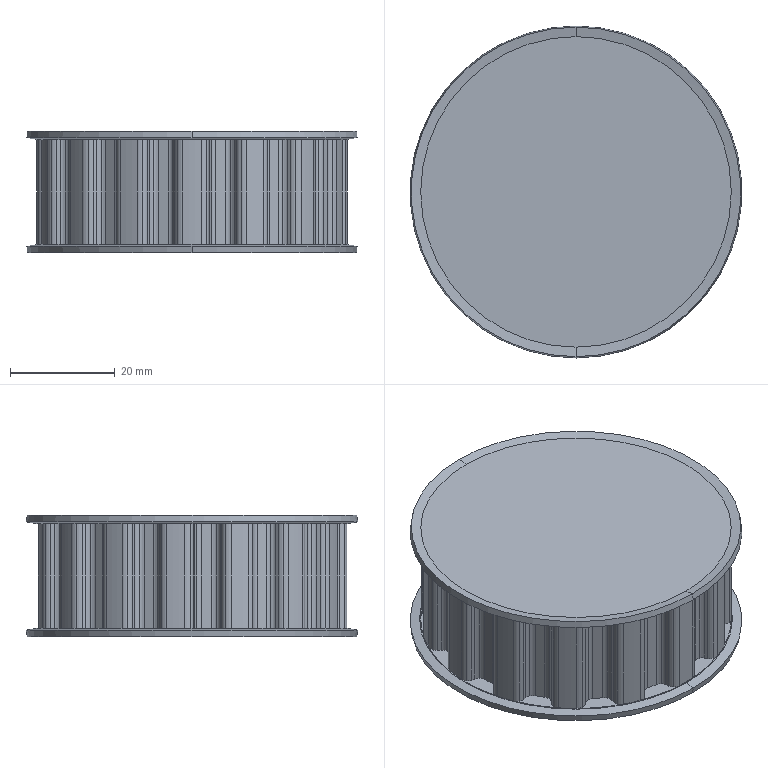Part | SolidWorks | features BaseBody 1 | 1 solid | 228 faces | box 63.33 x 63.33 x 23.179 mm | volume 58336 mm3 | cylinder 135 | plane 77 | cone 12 | torus 4 | commonest cylinder face diameters 3.2 x120 59.266 x15